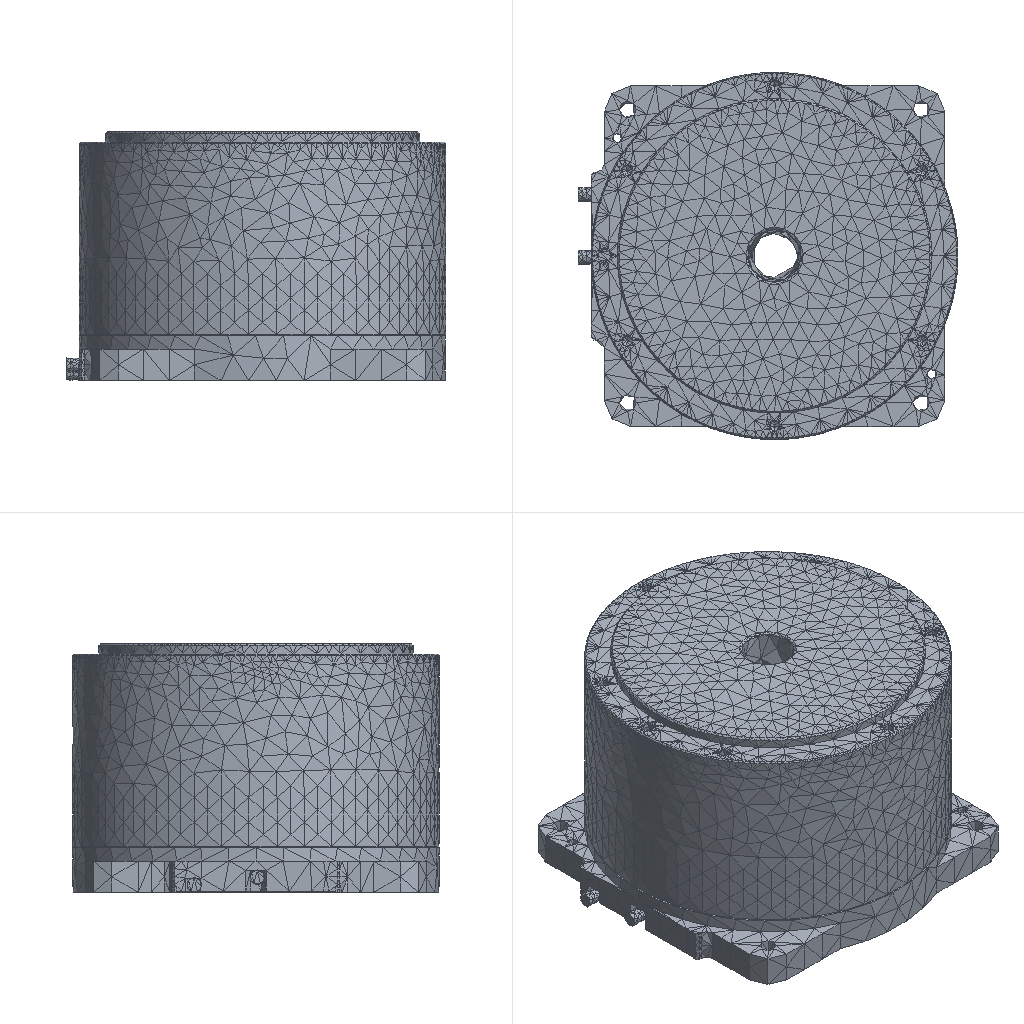Simulation study | ansys workbench
Ansys APDL input file, long lists of numbers shortened:
/batch
/config,noeldb,1     ! force off writing results to database
*get,_wallstrt,active,,time,wall
! ANSYS input file written by Workbench version 2022 R1
! File used for geometry attach:
/title,wbnew--____ (B5)
! ****** Begin Custom Load Command Snippet ******
/COM, ACT Extensions:
/COM,     LSDYNA, 2021.1
/COM,
! ****** End   Custom Load Command Snippet ******
*DIM,_wb_ProjectScratch_dir,string,248
_wb_ProjectScratch_dir(1) = ''
*DIM,_wb_SolverFiles_dir,string,248
_wb_SolverFiles_dir(1) = ''
*DIM,_wb_userfiles_dir,string,248
_wb_userfiles_dir(1) = ''
/com,--- Data in consistent NMM units. See Solving Units in the help system for more information.
/units,MPA
/nopr
/wb,file,start              !  signify a WB generated input file
/prep7
! Turn off shape checking because checks already performed inside WB mesher.
! See help system for more information.
SHPP,OFF,,NOWARN
/nolist
etcon,set             ! allow ANSYS to choose best KEYOP's for 180x elements, resets any applicable keyopt to MAPDL defaults
/com,*********** Nodes for the whole assembly ***********
nblock,3,,40216
(1i9,3e20.9e3)
        1    -6.000000000E+01     2.285569450E+01    -1.150000000E+01
! (36559 more lines like these left out)
-1
/com,*********** Nodes for all Remote Points ***********
nblock,3
(1i9,3e20.9e3)
    36561    -5.281372649E-16    -3.755781310E-03     3.700000029E+01
-1
/wb,elem,start            !  set before creation of elements
/com,*********** Elements for Body 1 "Assem3|1|1" ***********
et,1,187
eblock,19,solid,,4699
(19i9)
        1        1        1        1        0        0        0        0       10        0     1011     2049     2569     3307     3183     3846     6890     3853     3849
! (9397 more lines like these left out)
-1
/com,*********** Elements for Body 2 "Assem3|2|2" ***********
et,2,187
eblock,19,solid,,505
(19i9)
        2        2        2        2        0        0        0        0       10        0        1      139      159      171      167      879      967      882      881
! (1009 more lines like these left out)
-1
/com,*********** Elements for Body 3 "Assem3|2|2[2]" ***********
et,3,187
eblock,19,solid,,505
(19i9)
        3        3        3        3        0        0        0        0       10        0      506     1118     1138     1150     1146     1858     1946     1861     1860
! (1009 more lines like these left out)
-1
/com,*********** Elements for Body 4 "Assem1|3|3" ***********
et,4,187
eblock,19,solid,,14859
(19i9)
        4        4        4        4        0        0        0        0       10        0     5710    12826    14529    13819    13770    29270    34738    29267    29266
! (29717 more lines like these left out)
-1
/wb,elem,end               !  done creating elements
/com,*********** Send User Defined Coordinate System(s) ***********
csys,0
toffst,273.15,  ! Temperature offset from absolute zero
/com,*********** Set Reference Temperature ***********
tref,22.
/wb,mat,start              !  starting to send materials
/com,*********** Send Materials ***********
Temperature = 'TEMP' ! Temperature
MP,DENS,1,7.85e-09,	! tonne mm^-3
MP,ALPX,1,1.2e-05,	! C^-1
MP,C,1,434000000,	! mm^2 s^-2 C^-1
MP,KXX,1,60.5,	! tonne mm s^-3 C^-1
MP,RSVX,1,0.00017,	! ohm mm
MP,EX,1,200000,	! tonne s^-2 mm^-1
MP,NUXY,1,0.3,
MP,MURX,1,10000,
Temperature = 'TEMP' ! Temperature
MP,DENS,2,7.85e-09,	! tonne mm^-3
MP,ALPX,2,1.2e-05,	! C^-1
MP,C,2,434000000,	! mm^2 s^-2 C^-1
MP,KXX,2,60.5,	! tonne mm s^-3 C^-1
MP,RSVX,2,0.00017,	! ohm mm
MP,EX,2,200000,	! tonne s^-2 mm^-1
MP,NUXY,2,0.3,
MP,MURX,2,10000,
Temperature = 'TEMP' ! Temperature
MP,DENS,3,7.85e-09,	! tonne mm^-3
MP,ALPX,3,1.2e-05,	! C^-1
MP,C,3,434000000,	! mm^2 s^-2 C^-1
MP,KXX,3,60.5,	! tonne mm s^-3 C^-1
MP,RSVX,3,0.00017,	! ohm mm
MP,EX,3,200000,	! tonne s^-2 mm^-1
MP,NUXY,3,0.3,
MP,MURX,3,10000,
Temperature = 'TEMP' ! Temperature
MP,DENS,4,7.85e-09,	! tonne mm^-3
MP,ALPX,4,1.2e-05,	! C^-1
MP,C,4,434000000,	! mm^2 s^-2 C^-1
MP,KXX,4,60.5,	! tonne mm s^-3 C^-1
MP,RSVX,4,0.00017,	! ohm mm
MP,EX,4,200000,	! tonne s^-2 mm^-1
MP,NUXY,4,0.3,
MP,MURX,4,10000,
/wb,mat,end                !  done sending materials
!************************* Model Summary ********************
!Assem3|1|1,	结构钢,	matid,	1
!Assem3|2|2,	结构钢,	matid,	2
!Assem3|2|2[2],	结构钢,	matid,	3
!Assem1|3|3,	结构钢,	matid,	4
!************************* End Model Summary ********************
! get the diagonal of the bounding box. Needed later for other things
*get,_xmin,node,,mnloc,x
*get,_ymin,node,,mnloc,y
*get,_zmin,node,,mnloc,z
*get,_xmax,node,,mxloc,x
*get,_ymax,node,,mxloc,y
*get,_zmax,node,,mxloc,z
_ASMDIAG=(_xmax-_xmin)*(_xmax-_xmin)+(_ymax-_ymin)*(_ymax-_ymin)+(_zmax-_zmin)*(_zmax-_zmin)
_ASMDIAG=SQRT(_ASMDIAG)
/wb,contact,start          !  starting to send contact
/com,*********** Create Contact "接触区域" ***********
/com,            Real Constant Set For Above Contact Is 6 & 5
*set,tid,6
*set,cid,5
r,tid
r,cid
et,tid,170
et,cid,174
eblock,10,,,8
(15i9)
    29174        6        6        6        0     2358     2363     2359     2359     5791     5801     2359     5790
! (7 more lines like these left out)
-1
eblock,10,,,8
(15i9)
    29182        5        5        5        0     2358     2363     2359     2359     5791     5801     2359     5790
! (7 more lines like these left out)
-1
eblock,10,,,160
(15i9)
    29190        5        6        5        0        1       37       57       57      173      391       57      175
! (159 more lines like these left out)
-1
eblock,10,,,160
(15i9)
    29350        6        5        6        0        1       37       57       57      173      391       57      175
! (159 more lines like these left out)
-1
keyo,cid,8,2               ! auto create asymmetric contact (from Program Controlled setting)
keyo,cid,10,0              ! adjust contact stiffness each NR iteration (from Program Controlled setting)
keyo,cid,12,5              ! bonded always
keyo,cid,18,1              ! small sliding turned on by application
keyo,cid,2,0               ! augmented Lagrange (from Program Controlled setting)
keyo,cid,4,0               ! on Gauss point (from Program Controlled setting)
keyo,cid,9,1               ! ignore initial gaps/penetration
keyo,cid,7,0               ! No Prediction
rmod,tid,3,10.      ! FKN
rmod,tid,5,0.       ! ICONT
rmod,tid,6,0.       ! PINB
rmod,tid,10,0.      ! CNOF
rmod,tid,12,0.      ! FKT
rmod,tid,36,35      ! WB DSID
rmod,cid,3,10.      ! FKN
rmod,cid,5,0.       ! ICONT
rmod,cid,6,0.       ! PINB
rmod,cid,10,0.      ! CNOF
rmod,cid,12,0.      ! FKT
rmod,cid,36,35      ! WB DSID
/com,*********** Create Contact "接触区域 2" ***********
/com,            Real Constant Set For Above Contact Is 8 & 7
*set,tid,8
*set,cid,7
r,tid
r,cid
et,tid,170
et,cid,174
eblock,10,,,4
(15i9)
    29510        8        8        8        0     2369     2375     2370     2370     5881     5888     2370     5879
    29511        8        8        8        0     2370     2375     2374     2374     5888     5912     2374     5887
    29512        8        8        8        0     2369     2372     2375     2375     5880     5902     2375     5881
    29513        8        8        8        0     2368     2372     2369     2369     5877     5880     2369     5876
-1
eblock,10,,,4
(15i9)
    29514        7        7        7        0     2369     2375     2370     2370     5881     5888     2370     5879
    29515        7        7        7        0     2370     2375     2374     2374     5888     5912     2374     5887
    29516        7        7        7        0     2369     2372     2375     2375     5880     5902     2375     5881
    29517        7        7        7        0     2368     2372     2369     2369     5877     5880     2369     5876
-1
eblock,10,,,100
(15i9)
    29518        7        8        7        0      980     1016     1036     1036     1152     1370     1036     1154
! (99 more lines like these left out)
-1
eblock,10,,,100
(15i9)
    29618        8        7        8        0      980     1016     1036     1036     1152     1370     1036     1154
! (99 more lines like these left out)
-1
keyo,cid,8,2               ! auto create asymmetric contact (from Program Controlled setting)
keyo,cid,10,0              ! adjust contact stiffness each NR iteration (from Program Controlled setting)
keyo,cid,12,5              ! bonded always
keyo,cid,18,1              ! small sliding turned on by application
keyo,cid,2,0               ! augmented Lagrange (from Program Controlled setting)
keyo,cid,4,0               ! on Gauss point (from Program Controlled setting)
keyo,cid,9,1               ! ignore initial gaps/penetration
keyo,cid,7,0               ! No Prediction
rmod,tid,3,10.      ! FKN
rmod,tid,5,0.       ! ICONT
rmod,tid,6,0.       ! PINB
rmod,tid,10,0.      ! CNOF
rmod,tid,12,0.      ! FKT
rmod,tid,36,38      ! WB DSID
rmod,cid,3,10.      ! FKN
rmod,cid,5,0.       ! ICONT
rmod,cid,6,0.       ! PINB
rmod,cid,10,0.      ! CNOF
rmod,cid,12,0.      ! FKT
rmod,cid,36,38      ! WB DSID
/com,*********** Create Contact "接触区域 3" ***********
/com,            Real Constant Set For Above Contact Is 10 & 9
*set,tid,10
*set,cid,9
r,tid
r,cid
et,tid,170
et,cid,174
eblock,10,,,78
(15i9)
    29718       10       10       10        0     2014     2398     2397     2397     3659     6062     2397     3658
! (77 more lines like these left out)
-1
eblock,10,,,78
(15i9)
    29796        9        9        9        0     2014     2398     2397     2397     3659     6062     2397     3658
! (77 more lines like these left out)
-1
eblock,10,,,71
(15i9)
    29874        9       10        9        0    10415    13111    10416    10416    14755    14762    10416    14751
! (70 more lines like these left out)
-1
eblock,10,,,71
(15i9)
    29945       10        9       10        0    10415    13111    10416    10416    14755    14762    10416    14751
! (70 more lines like these left out)
-1
keyo,cid,8,2               ! auto create asymmetric contact (from Program Controlled setting)
keyo,cid,10,0              ! adjust contact stiffness each NR iteration (from Program Controlled setting)
keyo,cid,12,5              ! bonded always
keyo,cid,18,1              ! small sliding turned on by application
keyo,cid,2,0               ! augmented Lagrange (from Program Controlled setting)
keyo,cid,4,0               ! on Gauss point (from Program Controlled setting)
keyo,cid,9,1               ! ignore initial gaps/penetration
keyo,cid,7,0               ! No Prediction
rmod,tid,3,10.      ! FKN
rmod,tid,5,0.       ! ICONT
rmod,tid,6,0.       ! PINB
rmod,tid,10,0.      ! CNOF
rmod,tid,12,0.      ! FKT
rmod,tid,36,41      ! WB DSID
rmod,cid,3,10.      ! FKN
rmod,cid,5,0.       ! ICONT
rmod,cid,6,0.       ! PINB
rmod,cid,10,0.      ! CNOF
rmod,cid,12,0.      ! FKT
rmod,cid,36,41      ! WB DSID
nsel,all
esel,all
/wb,contact,end            !  done creating contacts
/golist
/wb,load,start             !  starting to send loads
CMBLOCK,_CM49_FIXEDSU,NODE,      650
(8i10)
      1959      1960      1961      1962      1963      1964      1965      1966
! (81 more lines like these left out)
/com,*********** Fixed Supports ***********
CMBLOCK,_FIXEDSU,NODE,      650
(8i10)
      1959      1960      1961      1962      1963      1964      1965      1966
! (81 more lines like these left out)
cmsel,s,_FIXEDSU
d,all,all
nsel,all
/com,*********** Create Remote Point "内部远程点" ***********
! -------- Remote Point Used by "力矩" --------
*set,tid,12
*set,cid,11
et,cid,174
et,tid,170
keyo,tid,2,1               ! Don't fix the pilot node
keyo,tid,4,111111
keyo,cid,12,5              ! Bonded Contact
keyo,cid,4,1               ! Deformable RBE3 style load
keyo,cid,2,2               ! MPC style contact
eblock,10,,,1637
(15i9)
    30016       11       11       11        0    10425    10426    12261    12261    14820    14831    12261    14825
! (1636 more lines like these left out)
-1
*set,_npilot,36561
_npilot52=_npilot
type,tid
mat ,cid
real,cid
tshape,pilo
en,31653,_npilot
tshape
/com,*********** Construct Moment Using Remote Attachment ***********
/gst,on,on
fini
*get,_numnode,node,0,count
*get,_numelem,elem,0,count
*get, _MAXELEMNUM, elem, 0, NUM, MAX
*get, _MAXNODENUM, node, 0, NUM, MAX
*get, _MAXELEMTYPE, etyp, 0, NUM, MAX
*get, _MAXREALCONST, real, 0, NUM, MAX
/go
/wb,load,end               !  done creating loads
/com,--- Number of total nodes = %_numnode%
/com,--- Number of contact elements = 2479
/com,--- Number of spring elements = 0
/com,--- Number of bearing elements = 0
/com,--- Number of solid elements = 20568
/com,--- Number of condensed parts = 0
/com,--- Number of total elements = %_numelem%
*get,_wallbsol,active,,time,wall
/com,****************************************************************************
/com,*************************    SOLUTION       ********************************
/com,****************************************************************************
/solu
antype,0                   ! static analysis
_thickRatio=  1     ! Ratio of thick parts in the model
eqsl,pcg,1e-8,,,,,,1
cntr,print,1               ! print out contact info and also make no initial contact an error
nldiag,cont,iter           ! print out contact info each equilibrium iteration
rescontrol,linear,last           ! Turn on restart files due to future eigen analysis intent
/com,****************************************************
/com,******************* SOLVE FOR LS 1 OF 1 ****************
nsel,s,node,,36561
f,all,mx,0.
f,all,my,0.
f,all,mz,5000.
nsel,all
/nopr
/gopr
nsub,1,1,1
time,1.
outres,erase
outres,all,none
outres,nsol,all,
outres,rsol,all
outres,eangl,all
outres,etmp,all
outres,veng,all
outres,strs,all,
outres,epel,all,
outres,eppl,all,
outres,cont,all,
! *********** WB SOLVE COMMAND ***********
! check interactive state
*get,ANSINTER_,active,,int
*if,ANSINTER_,ne,0,then
/eof
*endif
solve
/com *************** Write FE CONNECTORS *********
CEWRITE,file,ce,,INTE
/com,****************************************************
/com,*************** FINISHED SOLVE FOR LS 1 *************
*get,_wallasol,active,,time,wall
/nopr
*get,_numnode,node,0,count
*get,_numelem,elem,0,count
*get, _MAXELEMNUM, elem, 0, NUM, MAX
*get, _MAXNODENUM, node, 0, NUM, MAX,,,INTERNAL
*get, _MAXELEMTYPE, etyp, 0, NUM, MAX
*get, _MAXREALCONST, real, 0, NUM, MAX
/gopr
*get,_PCGITER,active,,solu,cgiter
/post1
xmlo,ENCODING,ISO-8859-1
xmlo,parm
/xml,parm,xml
fini
/gopr
*get,_walldone,active,,time,wall
_preptime=(_wallbsol-_wallstrt)*3600
_solvtime=(_wallasol-_wallbsol)*3600
_posttime=(_walldone-_wallasol)*3600
_totaltim=(_walldone-_wallstrt)*3600
*get,_dlbratio,active,0,solu,dlbr
*get,_combtime,active,0,solu,comb
*get,_ssmode,active,0,solu,ssmm
*get,_ndofs,active,0,solu,ndof
/com,--- Total number of nodes = %_numnode%
/com,--- Total number of elements = %_numelem%
/com,--- Element load balance ratio = %_dlbratio%
/com,--- Time to combine distributed files = %_combtime%
/com,--- Sparse memory mode = %_ssmode%
/com,--- Number of DOF = %_ndofs%
/wb,file,end               ! done with WB generated input